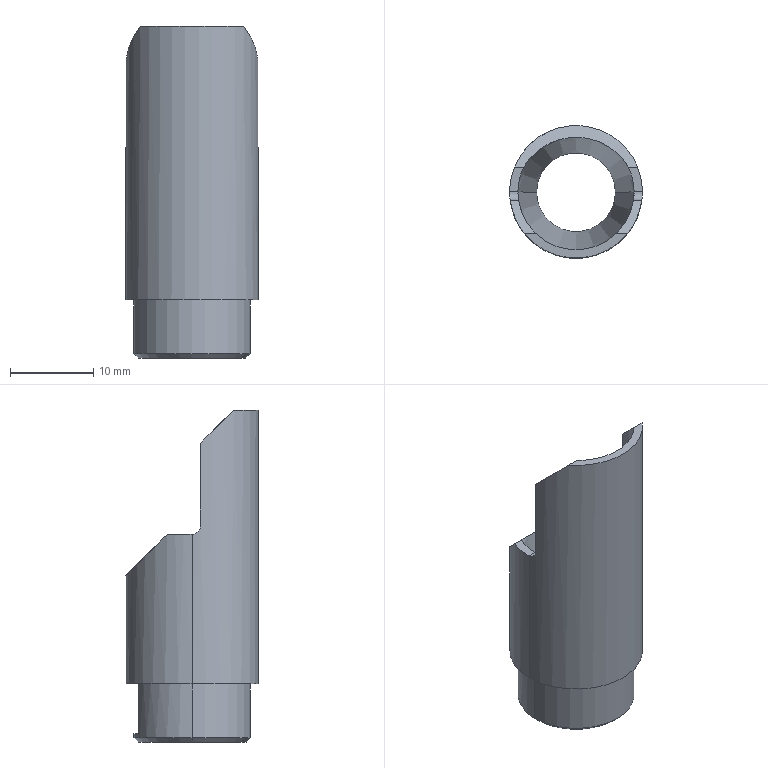Part | SolidWorks | features ICE 5, Chamfer 3, Extrusion 1, Fillet 1 | 1 solid | 25 faces | box 16 x 16 x 40 mm | volume 2380 mm3 | plane 12 | cylinder 9 | cone 4 | commonest cylinder face diameters 14 x3 2 x2 9.5 x2 16 x2
STEP:
#1=CARTESIAN_POINT('',(-4.75,0.,5.));
#2=VERTEX_POINT('',#1);
#3=CARTESIAN_POINT('',(4.75,0.,5.));
#4=VERTEX_POINT('',#3);
#5=CARTESIAN_POINT('',(0.,0.,5.));
#6=DIRECTION('',(0.,0.,1.));
#7=DIRECTION('',(1.,0.,0.));
#8=AXIS2_PLACEMENT_3D('',#5,#6,#7);
#9=CIRCLE('',#8,4.75);
#10=EDGE_CURVE('',#2,#4,#9,.T.);
#11=ORIENTED_EDGE('',*,*,#10,.F.);
#12=CARTESIAN_POINT('',(-7.,0.,25.));
#13=VERTEX_POINT('',#12);
#14=CARTESIAN_POINT('',(-4.75,0.,5.));
#15=DIRECTION('',(-0.1118,0.,0.9937));
#16=VECTOR('',#15,1000.);
#17=LINE('',#14,#16);
#18=EDGE_CURVE('',#2,#13,#17,.T.);
#19=ORIENTED_EDGE('',*,*,#18,.T.);
#20=CARTESIAN_POINT('',(7.,0.,25.));
#21=VERTEX_POINT('',#20);
#22=CARTESIAN_POINT('',(0.,0.,25.));
#23=DIRECTION('',(0.,0.,1.));
#24=DIRECTION('',(1.,0.,0.));
#25=AXIS2_PLACEMENT_3D('',#22,#23,#24);
#26=CIRCLE('',#25,7.);
#27=EDGE_CURVE('',#13,#21,#26,.T.);
#28=ORIENTED_EDGE('',*,*,#27,.T.);
#29=CARTESIAN_POINT('',(4.75,0.,5.));
#30=DIRECTION('',(0.1118,0.,0.9937));
#31=VECTOR('',#30,1000.);
#32=LINE('',#29,#31);
#33=EDGE_CURVE('',#4,#21,#32,.T.);
#34=ORIENTED_EDGE('',*,*,#33,.F.);
#35=EDGE_LOOP('',(#11,#19,#28,#34));
#36=FACE_OUTER_BOUND('',#35,.T.);
#37=CARTESIAN_POINT('',(0.,0.,5.));
#38=DIRECTION('',(0.,0.,1.));
#39=DIRECTION('',(1.,0.,0.));
#40=AXIS2_PLACEMENT_3D('',#37,#38,#39);
#41=CONICAL_SURFACE('',#40,4.75,0.112);
#42=ADVANCED_FACE('',(#36),#41,.F.);
#43=CARTESIAN_POINT('',(-6.5,0.,0.));
#44=VERTEX_POINT('',#43);
#45=CARTESIAN_POINT('',(6.5,0.,0.));
#46=VERTEX_POINT('',#45);
#47=CARTESIAN_POINT('',(0.,0.,0.));
#48=DIRECTION('',(0.,0.,-1.));
#49=DIRECTION('',(1.,0.,0.));
#50=AXIS2_PLACEMENT_3D('',#47,#48,#49);
#51=CIRCLE('',#50,6.5);
#52=EDGE_CURVE('',#44,#46,#51,.T.);
#53=ORIENTED_EDGE('',*,*,#52,.F.);
#54=CARTESIAN_POINT('',(-7.,0.,0.5));
#55=VERTEX_POINT('',#54);
#56=CARTESIAN_POINT('',(-6.5,0.,0.));
#57=DIRECTION('',(-0.7071,0.,0.7071));
#58=VECTOR('',#57,1000.);
#59=LINE('',#56,#58);
#60=EDGE_CURVE('',#44,#55,#59,.T.);
#61=ORIENTED_EDGE('',*,*,#60,.T.);
#62=CARTESIAN_POINT('',(7.,0.,0.5));
#63=VERTEX_POINT('',#62);
#64=CARTESIAN_POINT('',(0.,0.,0.5));
#65=DIRECTION('',(0.,0.,1.));
#66=DIRECTION('',(1.,0.,0.));
#67=AXIS2_PLACEMENT_3D('',#64,#65,#66);
#68=CIRCLE('',#67,7.);
#69=EDGE_CURVE('',#63,#55,#68,.T.);
#70=ORIENTED_EDGE('',*,*,#69,.F.);
#71=CARTESIAN_POINT('',(6.5,0.,0.));
#72=DIRECTION('',(0.7071,0.,0.7071));
#73=VECTOR('',#72,1000.);
#74=LINE('',#71,#73);
#75=EDGE_CURVE('',#46,#63,#74,.T.);
#76=ORIENTED_EDGE('',*,*,#75,.F.);
#77=EDGE_LOOP('',(#53,#61,#70,#76));
#78=FACE_OUTER_BOUND('',#77,.T.);
#79=CARTESIAN_POINT('',(0.,0.,0.));
#80=DIRECTION('',(0.,0.,1.));
#81=DIRECTION('',(1.,0.,0.));
#82=AXIS2_PLACEMENT_3D('',#79,#80,#81);
#83=CONICAL_SURFACE('',#82,6.5,0.7854);
#84=ADVANCED_FACE('',(#78),#83,.T.);
#85=CARTESIAN_POINT('',(7.416,3.,25.));
#86=VERTEX_POINT('',#85);
#87=CARTESIAN_POINT('',(8.,0.,25.));
#88=VERTEX_POINT('',#87);
#89=CARTESIAN_POINT('',(0.,0.,25.));
#90=DIRECTION('',(0.,0.,-1.));
#91=DIRECTION('',(-1.,0.,0.));
#92=AXIS2_PLACEMENT_3D('',#89,#90,#91);
#93=CIRCLE('',#92,8.);
#94=EDGE_CURVE('',#86,#88,#93,.T.);
#95=ORIENTED_EDGE('',*,*,#94,.T.);
#96=CARTESIAN_POINT('',(8.,0.,7.));
#97=VERTEX_POINT('',#96);
#98=CARTESIAN_POINT('',(8.,0.,40.));
#99=DIRECTION('',(0.,0.,-1.));
#100=VECTOR('',#99,1000.);
#101=LINE('',#98,#100);
#102=EDGE_CURVE('',#88,#97,#101,.T.);
#103=ORIENTED_EDGE('',*,*,#102,.T.);
#104=CARTESIAN_POINT('',(-8.,0.,7.));
#105=VERTEX_POINT('',#104);
#106=CARTESIAN_POINT('',(0.,0.,7.));
#107=DIRECTION('',(0.,0.,-1.));
#108=DIRECTION('',(-1.,0.,0.));
#109=AXIS2_PLACEMENT_3D('',#106,#107,#108);
#110=CIRCLE('',#109,8.);
#111=EDGE_CURVE('',#105,#97,#110,.T.);
#112=ORIENTED_EDGE('',*,*,#111,.F.);
#113=CARTESIAN_POINT('',(-8.,0.,25.));
#114=VERTEX_POINT('',#113);
#115=CARTESIAN_POINT('',(-8.,0.,40.));
#116=DIRECTION('',(0.,0.,-1.));
#117=VECTOR('',#116,1000.);
#118=LINE('',#115,#117);
#119=EDGE_CURVE('',#114,#105,#118,.T.);
#120=ORIENTED_EDGE('',*,*,#119,.F.);
#121=CARTESIAN_POINT('',(-7.416,3.,25.));
#122=VERTEX_POINT('',#121);
#123=CARTESIAN_POINT('',(0.,0.,25.));
#124=DIRECTION('',(0.,0.,-1.));
#125=DIRECTION('',(-1.,0.,0.));
#126=AXIS2_PLACEMENT_3D('',#123,#124,#125);
#127=CIRCLE('',#126,8.);
#128=EDGE_CURVE('',#114,#122,#127,.T.);
#129=ORIENTED_EDGE('',*,*,#128,.T.);
#130=CARTESIAN_POINT('',(-7.416,3.,25.));
#131=CARTESIAN_POINT('',(-4.238,10.857,17.143));
#132=CARTESIAN_POINT('',(4.238,10.857,17.143));
#133=CARTESIAN_POINT('',(7.416,3.,25.));
#134=(BOUNDED_CURVE()B_SPLINE_CURVE(3,(#130,#131,#132,#133),.UNSPECIFIED.,.F.,.F.)B_SPLINE_CURVE_WITH_KNOTS((4,4),(5.097,7.47),.UNSPECIFIED.)CURVE()GEOMETRIC_REPRESENTATION_ITEM()RATIONAL_B_SPLINE_CURVE((1.,0.5833,0.5833,1.))REPRESENTATION_ITEM(''));
#135=EDGE_CURVE('',#122,#86,#134,.T.);
#136=ORIENTED_EDGE('',*,*,#135,.T.);
#137=EDGE_LOOP('',(#95,#103,#112,#120,#129,#136));
#138=FACE_OUTER_BOUND('',#137,.T.);
#139=CARTESIAN_POINT('',(0.,0.,40.));
#140=DIRECTION('',(0.,0.,-1.));
#141=DIRECTION('',(-1.,0.,0.));
#142=AXIS2_PLACEMENT_3D('',#139,#140,#141);
#143=CYLINDRICAL_SURFACE('',#142,8.);
#144=ADVANCED_FACE('',(#138),#143,.T.);
#145=ORIENTED_EDGE('',*,*,#10,.T.);
#146=CARTESIAN_POINT('',(4.75,0.,0.));
#147=VERTEX_POINT('',#146);
#148=CARTESIAN_POINT('',(4.75,0.,40.));
#149=DIRECTION('',(0.,0.,-1.));
#150=VECTOR('',#149,1000.);
#151=LINE('',#148,#150);
#152=EDGE_CURVE('',#4,#147,#151,.T.);
#153=ORIENTED_EDGE('',*,*,#152,.T.);
#154=CARTESIAN_POINT('',(-4.75,0.,0.));
#155=VERTEX_POINT('',#154);
#156=CARTESIAN_POINT('',(0.,0.,0.));
#157=DIRECTION('',(0.,0.,1.));
#158=DIRECTION('',(1.,0.,0.));
#159=AXIS2_PLACEMENT_3D('',#156,#157,#158);
#160=CIRCLE('',#159,4.75);
#161=EDGE_CURVE('',#155,#147,#160,.T.);
#162=ORIENTED_EDGE('',*,*,#161,.F.);
#163=CARTESIAN_POINT('',(-4.75,0.,40.));
#164=DIRECTION('',(0.,0.,-1.));
#165=VECTOR('',#164,1000.);
#166=LINE('',#163,#165);
#167=EDGE_CURVE('',#2,#155,#166,.T.);
#168=ORIENTED_EDGE('',*,*,#167,.F.);
#169=EDGE_LOOP('',(#145,#153,#162,#168));
#170=FACE_OUTER_BOUND('',#169,.T.);
#171=CARTESIAN_POINT('',(0.,0.,40.));
#172=DIRECTION('',(0.,0.,-1.));
#173=DIRECTION('',(-1.,0.,0.));
#174=AXIS2_PLACEMENT_3D('',#171,#172,#173);
#175=CYLINDRICAL_SURFACE('',#174,4.75);
#176=ADVANCED_FACE('',(#170),#175,.F.);
#177=CARTESIAN_POINT('',(2.598,6.5,7.));
#178=VERTEX_POINT('',#177);
#179=CARTESIAN_POINT('',(7.,0.,7.));
#180=VERTEX_POINT('',#179);
#181=CARTESIAN_POINT('',(0.,0.,7.));
#182=DIRECTION('',(0.,0.,-1.));
#183=DIRECTION('',(-1.,0.,0.));
#184=AXIS2_PLACEMENT_3D('',#181,#182,#183);
#185=CIRCLE('',#184,7.);
#186=EDGE_CURVE('',#178,#180,#185,.T.);
#187=ORIENTED_EDGE('',*,*,#186,.T.);
#188=CARTESIAN_POINT('',(7.,0.,7.));
#189=DIRECTION('',(0.,0.,-1.));
#190=VECTOR('',#189,1000.);
#191=LINE('',#188,#190);
#192=EDGE_CURVE('',#180,#63,#191,.T.);
#193=ORIENTED_EDGE('',*,*,#192,.T.);
#194=ORIENTED_EDGE('',*,*,#69,.T.);
#195=CARTESIAN_POINT('',(-7.,0.,7.));
#196=VERTEX_POINT('',#195);
#197=CARTESIAN_POINT('',(-7.,0.,7.));
#198=DIRECTION('',(0.,0.,-1.));
#199=VECTOR('',#198,1000.);
#200=LINE('',#197,#199);
#201=EDGE_CURVE('',#196,#55,#200,.T.);
#202=ORIENTED_EDGE('',*,*,#201,.F.);
#203=CARTESIAN_POINT('',(-2.598,6.5,7.));
#204=VERTEX_POINT('',#203);
#205=CARTESIAN_POINT('',(0.,0.,7.));
#206=DIRECTION('',(0.,0.,-1.));
#207=DIRECTION('',(-1.,0.,0.));
#208=AXIS2_PLACEMENT_3D('',#205,#206,#207);
#209=CIRCLE('',#208,7.);
#210=EDGE_CURVE('',#196,#204,#209,.T.);
#211=ORIENTED_EDGE('',*,*,#210,.T.);
#212=CARTESIAN_POINT('',(-2.598,6.5,1.));
#213=VERTEX_POINT('',#212);
#214=CARTESIAN_POINT('',(-2.598,6.5,1.));
#215=DIRECTION('',(0.,0.,1.));
#216=VECTOR('',#215,1000.);
#217=LINE('',#214,#216);
#218=EDGE_CURVE('',#213,#204,#217,.T.);
#219=ORIENTED_EDGE('',*,*,#218,.F.);
#220=CARTESIAN_POINT('',(2.598,6.5,1.));
#221=VERTEX_POINT('',#220);
#222=CARTESIAN_POINT('',(0.,0.,1.));
#223=DIRECTION('',(0.,0.,-1.));
#224=DIRECTION('',(-1.,0.,0.));
#225=AXIS2_PLACEMENT_3D('',#222,#223,#224);
#226=CIRCLE('',#225,7.);
#227=EDGE_CURVE('',#213,#221,#226,.T.);
#228=ORIENTED_EDGE('',*,*,#227,.T.);
#229=CARTESIAN_POINT('',(2.598,6.5,1.));
#230=DIRECTION('',(0.,0.,1.));
#231=VECTOR('',#230,1000.);
#232=LINE('',#229,#231);
#233=EDGE_CURVE('',#221,#178,#232,.T.);
#234=ORIENTED_EDGE('',*,*,#233,.T.);
#235=EDGE_LOOP('',(#187,#193,#194,#202,#211,#219,#228,#234));
#236=FACE_OUTER_BOUND('',#235,.T.);
#237=CARTESIAN_POINT('',(0.,0.,7.));
#238=DIRECTION('',(0.,0.,-1.));
#239=DIRECTION('',(-1.,0.,0.));
#240=AXIS2_PLACEMENT_3D('',#237,#238,#239);
#241=CYLINDRICAL_SURFACE('',#240,7.);
#242=ADVANCED_FACE('',(#236),#241,.T.);
#243=ORIENTED_EDGE('',*,*,#192,.F.);
#244=CARTESIAN_POINT('',(0.,0.,7.));
#245=DIRECTION('',(0.,0.,-1.));
#246=DIRECTION('',(-1.,0.,0.));
#247=AXIS2_PLACEMENT_3D('',#244,#245,#246);
#248=CIRCLE('',#247,7.);
#249=EDGE_CURVE('',#180,#196,#248,.T.);
#250=ORIENTED_EDGE('',*,*,#249,.T.);
#251=ORIENTED_EDGE('',*,*,#201,.T.);
#252=CARTESIAN_POINT('',(0.,0.,0.5));
#253=DIRECTION('',(0.,0.,1.));
#254=DIRECTION('',(1.,0.,0.));
#255=AXIS2_PLACEMENT_3D('',#252,#253,#254);
#256=CIRCLE('',#255,7.);
#257=EDGE_CURVE('',#55,#63,#256,.T.);
#258=ORIENTED_EDGE('',*,*,#257,.T.);
#259=EDGE_LOOP('',(#243,#250,#251,#258));
#260=FACE_OUTER_BOUND('',#259,.T.);
#261=CARTESIAN_POINT('',(0.,0.,7.));
#262=DIRECTION('',(0.,0.,-1.));
#263=DIRECTION('',(-1.,0.,0.));
#264=AXIS2_PLACEMENT_3D('',#261,#262,#263);
#265=CYLINDRICAL_SURFACE('',#264,7.);
#266=ADVANCED_FACE('',(#260),#265,.T.);
#267=ORIENTED_EDGE('',*,*,#128,.F.);
#268=CARTESIAN_POINT('',(0.,0.,25.));
#269=DIRECTION('',(1.,0.,0.));
#270=VECTOR('',#269,1000.);
#271=LINE('',#268,#270);
#272=EDGE_CURVE('',#114,#13,#271,.T.);
#273=ORIENTED_EDGE('',*,*,#272,.T.);
#274=CARTESIAN_POINT('',(-6.325,3.,25.));
#275=VERTEX_POINT('',#274);
#276=CARTESIAN_POINT('',(0.,0.,25.));
#277=DIRECTION('',(0.,0.,-1.));
#278=DIRECTION('',(1.,0.,0.));
#279=AXIS2_PLACEMENT_3D('',#276,#277,#278);
#280=CIRCLE('',#279,7.);
#281=EDGE_CURVE('',#13,#275,#280,.T.);
#282=ORIENTED_EDGE('',*,*,#281,.T.);
#283=CARTESIAN_POINT('',(-8.,3.,25.));
#284=DIRECTION('',(1.,0.,0.));
#285=VECTOR('',#284,1000.);
#286=LINE('',#283,#285);
#287=EDGE_CURVE('',#122,#275,#286,.T.);
#288=ORIENTED_EDGE('',*,*,#287,.F.);
#289=EDGE_LOOP('',(#267,#273,#282,#288));
#290=FACE_OUTER_BOUND('',#289,.T.);
#291=CARTESIAN_POINT('',(0.,0.,25.));
#292=DIRECTION('',(0.,0.,1.));
#293=DIRECTION('',(1.,0.,0.));
#294=AXIS2_PLACEMENT_3D('',#291,#292,#293);
#295=PLANE('',#294);
#296=ADVANCED_FACE('',(#290),#295,.T.);
#297=ORIENTED_EDGE('',*,*,#152,.F.);
#298=CARTESIAN_POINT('',(0.,0.,5.));
#299=DIRECTION('',(0.,0.,1.));
#300=DIRECTION('',(1.,0.,0.));
#301=AXIS2_PLACEMENT_3D('',#298,#299,#300);
#302=CIRCLE('',#301,4.75);
#303=EDGE_CURVE('',#4,#2,#302,.T.);
#304=ORIENTED_EDGE('',*,*,#303,.T.);
#305=ORIENTED_EDGE('',*,*,#167,.T.);
#306=CARTESIAN_POINT('',(0.,0.,0.));
#307=DIRECTION('',(0.,0.,1.));
#308=DIRECTION('',(1.,0.,0.));
#309=AXIS2_PLACEMENT_3D('',#306,#307,#308);
#310=CIRCLE('',#309,4.75);
#311=EDGE_CURVE('',#147,#155,#310,.T.);
#312=ORIENTED_EDGE('',*,*,#311,.F.);
#313=EDGE_LOOP('',(#297,#304,#305,#312));
#314=FACE_OUTER_BOUND('',#313,.T.);
#315=CARTESIAN_POINT('',(0.,0.,40.));
#316=DIRECTION('',(0.,0.,-1.));
#317=DIRECTION('',(-1.,0.,0.));
#318=AXIS2_PLACEMENT_3D('',#315,#316,#317);
#319=CYLINDRICAL_SURFACE('',#318,4.75);
#320=ADVANCED_FACE('',(#314),#319,.F.);
#321=CARTESIAN_POINT('',(0.,0.,0.));
#322=DIRECTION('',(0.,0.,-1.));
#323=DIRECTION('',(1.,0.,0.));
#324=AXIS2_PLACEMENT_3D('',#321,#322,#323);
#325=CIRCLE('',#324,6.5);
#326=EDGE_CURVE('',#46,#44,#325,.T.);
#327=ORIENTED_EDGE('',*,*,#326,.T.);
#328=ORIENTED_EDGE('',*,*,#52,.T.);
#329=EDGE_LOOP('',(#327,#328));
#330=FACE_OUTER_BOUND('',#329,.T.);
#331=ORIENTED_EDGE('',*,*,#161,.T.);
#332=ORIENTED_EDGE('',*,*,#311,.T.);
#333=EDGE_LOOP('',(#331,#332));
#334=FACE_BOUND('',#333,.T.);
#335=CARTESIAN_POINT('',(0.,0.,0.));
#336=DIRECTION('',(0.,0.,1.));
#337=DIRECTION('',(1.,0.,0.));
#338=AXIS2_PLACEMENT_3D('',#335,#336,#337);
#339=PLANE('',#338);
#340=ADVANCED_FACE('',(#330,#334),#339,.F.);
#341=ORIENTED_EDGE('',*,*,#102,.F.);
#342=CARTESIAN_POINT('',(7.937,-1.,26.));
#343=VERTEX_POINT('',#342);
#344=CARTESIAN_POINT('',(8.,0.,25.));
#345=CARTESIAN_POINT('',(8.,-0.1322,25.));
#346=CARTESIAN_POINT('',(7.997,-0.2619,25.026));
#347=CARTESIAN_POINT('',(7.985,-0.5039,25.126));
#348=CARTESIAN_POINT('',(7.977,-0.6147,25.201));
#349=CARTESIAN_POINT('',(7.952,-0.8911,25.477));
#350=CARTESIAN_POINT('',(7.937,-1.,25.736));
#351=CARTESIAN_POINT('',(7.937,-1.,26.));
#352=B_SPLINE_CURVE_WITH_KNOTS('',3,(#344,#345,#346,#347,#348,#349,#350,#351),.UNSPECIFIED.,.F.,.F.,(4,2,2,4),(0.,0.0003909,0.0007818,0.001564),.UNSPECIFIED.);
#353=EDGE_CURVE('',#88,#343,#352,.T.);
#354=ORIENTED_EDGE('',*,*,#353,.T.);
#355=CARTESIAN_POINT('',(7.937,-1.,36.));
#356=VERTEX_POINT('',#355);
#357=CARTESIAN_POINT('',(7.937,-1.,40.));
#358=DIRECTION('',(0.,0.,1.));
#359=VECTOR('',#358,1000.);
#360=LINE('',#357,#359);
#361=EDGE_CURVE('',#343,#356,#360,.T.);
#362=ORIENTED_EDGE('',*,*,#361,.T.);
#363=CARTESIAN_POINT('',(6.245,-5.,40.));
#364=VERTEX_POINT('',#363);
#365=CARTESIAN_POINT('',(7.937,-1.,36.));
#366=CARTESIAN_POINT('',(7.752,-2.473,37.473));
#367=CARTESIAN_POINT('',(7.173,-3.841,38.841));
#368=CARTESIAN_POINT('',(6.245,-5.,40.));
#369=(BOUNDED_CURVE()B_SPLINE_CURVE(3,(#365,#366,#367,#368),.UNSPECIFIED.,.F.,.F.)B_SPLINE_CURVE_WITH_KNOTS((4,4),(1.696,2.246),.UNSPECIFIED.)CURVE()GEOMETRIC_REPRESENTATION_ITEM()RATIONAL_B_SPLINE_CURVE((1.,0.975,0.975,1.))REPRESENTATION_ITEM(''));
#370=EDGE_CURVE('',#356,#364,#369,.T.);
#371=ORIENTED_EDGE('',*,*,#370,.T.);
#372=CARTESIAN_POINT('',(-6.245,-5.,40.));
#373=VERTEX_POINT('',#372);
#374=CARTESIAN_POINT('',(0.,0.,40.));
#375=DIRECTION('',(0.,0.,1.));
#376=DIRECTION('',(1.,0.,0.));
#377=AXIS2_PLACEMENT_3D('',#374,#375,#376);
#378=CIRCLE('',#377,8.);
#379=EDGE_CURVE('',#373,#364,#378,.T.);
#380=ORIENTED_EDGE('',*,*,#379,.F.);
#381=CARTESIAN_POINT('',(-7.937,-1.,36.));
#382=VERTEX_POINT('',#381);
#383=CARTESIAN_POINT('',(-6.245,-5.,40.));
#384=CARTESIAN_POINT('',(-7.173,-3.841,38.841));
#385=CARTESIAN_POINT('',(-7.752,-2.473,37.473));
#386=CARTESIAN_POINT('',(-7.937,-1.,36.));
#387=(BOUNDED_CURVE()B_SPLINE_CURVE(3,(#383,#384,#385,#386),.UNSPECIFIED.,.F.,.F.)B_SPLINE_CURVE_WITH_KNOTS((4,4),(4.037,4.587),.UNSPECIFIED.)CURVE()GEOMETRIC_REPRESENTATION_ITEM()RATIONAL_B_SPLINE_CURVE((1.,0.975,0.975,1.))REPRESENTATION_ITEM(''));
#388=EDGE_CURVE('',#373,#382,#387,.T.);
#389=ORIENTED_EDGE('',*,*,#388,.T.);
#390=CARTESIAN_POINT('',(-7.937,-1.,26.));
#391=VERTEX_POINT('',#390);
#392=CARTESIAN_POINT('',(-7.937,-1.,40.));
#393=DIRECTION('',(0.,0.,-1.));
#394=VECTOR('',#393,1000.);
#395=LINE('',#392,#394);
#396=EDGE_CURVE('',#382,#391,#395,.T.);
#397=ORIENTED_EDGE('',*,*,#396,.T.);
#398=CARTESIAN_POINT('',(-7.937,-1.,26.));
#399=CARTESIAN_POINT('',(-7.937,-1.,25.868));
#400=CARTESIAN_POINT('',(-7.941,-0.9739,25.738));
#401=CARTESIAN_POINT('',(-7.952,-0.8736,25.496));
#402=CARTESIAN_POINT('',(-7.96,-0.7994,25.385));
#403=CARTESIAN_POINT('',(-7.985,-0.5232,25.109));
#404=CARTESIAN_POINT('',(-8.,-0.2644,25.));
#405=CARTESIAN_POINT('',(-8.,0.,25.));
#406=B_SPLINE_CURVE_WITH_KNOTS('',3,(#398,#399,#400,#401,#402,#403,#404,#405),.UNSPECIFIED.,.F.,.F.,(4,2,2,4),(0.,0.0003909,0.0007818,0.001564),.UNSPECIFIED.);
#407=EDGE_CURVE('',#391,#114,#406,.T.);
#408=ORIENTED_EDGE('',*,*,#407,.T.);
#409=ORIENTED_EDGE('',*,*,#119,.T.);
#410=CARTESIAN_POINT('',(0.,0.,7.));
#411=DIRECTION('',(0.,0.,-1.));
#412=DIRECTION('',(-1.,0.,0.));
#413=AXIS2_PLACEMENT_3D('',#410,#411,#412);
#414=CIRCLE('',#413,8.);
#415=EDGE_CURVE('',#97,#105,#414,.T.);
#416=ORIENTED_EDGE('',*,*,#415,.F.);
#417=EDGE_LOOP('',(#341,#354,#362,#371,#380,#389,#397,#408,#409,#416));
#418=FACE_OUTER_BOUND('',#417,.T.);
#419=CARTESIAN_POINT('',(0.,0.,40.));
#420=DIRECTION('',(0.,0.,-1.));
#421=DIRECTION('',(-1.,0.,0.));
#422=AXIS2_PLACEMENT_3D('',#419,#420,#421);
#423=CYLINDRICAL_SURFACE('',#422,8.);
#424=ADVANCED_FACE('',(#418),#423,.T.);
#425=ORIENTED_EDGE('',*,*,#379,.T.);
#426=CARTESIAN_POINT('',(4.899,-5.,40.));
#427=VERTEX_POINT('',#426);
#428=CARTESIAN_POINT('',(6.928,-5.,40.));
#429=DIRECTION('',(-1.,0.,0.));
#430=VECTOR('',#429,1000.);
#431=LINE('',#428,#430);
#432=EDGE_CURVE('',#364,#427,#431,.T.);
#433=ORIENTED_EDGE('',*,*,#432,.T.);
#434=CARTESIAN_POINT('',(-4.899,-5.,40.));
#435=VERTEX_POINT('',#434);
#436=CARTESIAN_POINT('',(0.,0.,40.));
#437=DIRECTION('',(0.,0.,1.));
#438=DIRECTION('',(1.,0.,0.));
#439=AXIS2_PLACEMENT_3D('',#436,#437,#438);
#440=CIRCLE('',#439,7.);
#441=EDGE_CURVE('',#435,#427,#440,.T.);
#442=ORIENTED_EDGE('',*,*,#441,.F.);
#443=CARTESIAN_POINT('',(-7.937,-5.,40.));
#444=DIRECTION('',(-1.,0.,0.));
#445=VECTOR('',#444,1000.);
#446=LINE('',#443,#445);
#447=EDGE_CURVE('',#435,#373,#446,.T.);
#448=ORIENTED_EDGE('',*,*,#447,.T.);
#449=EDGE_LOOP('',(#425,#433,#442,#448));
#450=FACE_OUTER_BOUND('',#449,.T.);
#451=CARTESIAN_POINT('',(0.,0.,40.));
#452=DIRECTION('',(0.,0.,1.));
#453=DIRECTION('',(1.,0.,0.));
#454=AXIS2_PLACEMENT_3D('',#451,#452,#453);
#455=PLANE('',#454);
#456=ADVANCED_FACE('',(#450),#455,.T.);
#457=ORIENTED_EDGE('',*,*,#186,.F.);
#458=CARTESIAN_POINT('',(2.598,6.5,7.));
#459=DIRECTION('',(-1.,0.,0.));
#460=VECTOR('',#459,1000.);
#461=LINE('',#458,#460);
#462=EDGE_CURVE('',#178,#204,#461,.T.);
#463=ORIENTED_EDGE('',*,*,#462,.T.);
#464=ORIENTED_EDGE('',*,*,#210,.F.);
#465=ORIENTED_EDGE('',*,*,#249,.F.);
#466=EDGE_LOOP('',(#457,#463,#464,#465));
#467=FACE_BOUND('',#466,.T.);
#468=ORIENTED_EDGE('',*,*,#111,.T.);
#469=ORIENTED_EDGE('',*,*,#415,.T.);
#470=EDGE_LOOP('',(#468,#469));
#471=FACE_OUTER_BOUND('',#470,.T.);
#472=CARTESIAN_POINT('',(0.,0.,7.));
#473=DIRECTION('',(0.,0.,-1.));
#474=DIRECTION('',(-1.,0.,0.));
#475=AXIS2_PLACEMENT_3D('',#472,#473,#474);
#476=PLANE('',#475);
#477=ADVANCED_FACE('',(#467,#471),#476,.T.);
#478=ORIENTED_EDGE('',*,*,#60,.F.);
#479=ORIENTED_EDGE('',*,*,#326,.F.);
#480=ORIENTED_EDGE('',*,*,#75,.T.);
#481=ORIENTED_EDGE('',*,*,#257,.F.);
#482=EDGE_LOOP('',(#478,#479,#480,#481));
#483=FACE_OUTER_BOUND('',#482,.T.);
#484=CARTESIAN_POINT('',(0.,0.,0.));
#485=DIRECTION('',(0.,0.,1.));
#486=DIRECTION('',(1.,0.,0.));
#487=AXIS2_PLACEMENT_3D('',#484,#485,#486);
#488=CONICAL_SURFACE('',#487,6.5,0.7854);
#489=ADVANCED_FACE('',(#483),#488,.T.);
#490=ORIENTED_EDGE('',*,*,#441,.T.);
#491=CARTESIAN_POINT('',(6.928,-1.,36.));
#492=VERTEX_POINT('',#491);
#493=CARTESIAN_POINT('',(4.899,-5.,40.));
#494=CARTESIAN_POINT('',(6.006,-3.916,38.916));
#495=CARTESIAN_POINT('',(6.707,-2.534,37.534));
#496=CARTESIAN_POINT('',(6.928,-1.,36.));
#497=(BOUNDED_CURVE()B_SPLINE_CURVE(3,(#493,#494,#495,#496),.UNSPECIFIED.,.F.,.F.)B_SPLINE_CURVE_WITH_KNOTS((4,4),(0.7752,1.427),.UNSPECIFIED.)CURVE()GEOMETRIC_REPRESENTATION_ITEM()RATIONAL_B_SPLINE_CURVE((1.,0.9649,0.9649,1.))REPRESENTATION_ITEM(''));
#498=EDGE_CURVE('',#427,#492,#497,.T.);
#499=ORIENTED_EDGE('',*,*,#498,.T.);
#500=CARTESIAN_POINT('',(6.928,-1.,26.));
#501=VERTEX_POINT('',#500);
#502=CARTESIAN_POINT('',(6.928,-1.,25.));
#503=DIRECTION('',(0.,0.,-1.));
#504=VECTOR('',#503,1000.);
#505=LINE('',#502,#504);
#506=EDGE_CURVE('',#492,#501,#505,.T.);
#507=ORIENTED_EDGE('',*,*,#506,.T.);
#508=CARTESIAN_POINT('',(6.928,-1.,26.));
#509=CARTESIAN_POINT('',(6.928,-1.,25.868));
#510=CARTESIAN_POINT('',(6.932,-0.9739,25.738));
#511=CARTESIAN_POINT('',(6.945,-0.8736,25.496));
#512=CARTESIAN_POINT('',(6.955,-0.7994,25.385));
#513=CARTESIAN_POINT('',(6.983,-0.5233,25.109));
#514=CARTESIAN_POINT('',(7.,-0.2645,25.));
#515=CARTESIAN_POINT('',(7.,0.,25.));
#516=B_SPLINE_CURVE_WITH_KNOTS('',3,(#508,#509,#510,#511,#512,#513,#514,#515),.UNSPECIFIED.,.F.,.F.,(4,2,2,4),(0.,0.000391,0.0007821,0.001564),.UNSPECIFIED.);
#517=EDGE_CURVE('',#501,#21,#516,.T.);
#518=ORIENTED_EDGE('',*,*,#517,.T.);
#519=ORIENTED_EDGE('',*,*,#27,.F.);
#520=CARTESIAN_POINT('',(-6.928,-1.,26.));
#521=VERTEX_POINT('',#520);
#522=CARTESIAN_POINT('',(-7.,0.,25.));
#523=CARTESIAN_POINT('',(-7.,-0.1322,25.));
#524=CARTESIAN_POINT('',(-6.996,-0.262,25.026));
#525=CARTESIAN_POINT('',(-6.983,-0.504,25.126));
#526=CARTESIAN_POINT('',(-6.974,-0.6148,25.201));
#527=CARTESIAN_POINT('',(-6.946,-0.8911,25.477));
#528=CARTESIAN_POINT('',(-6.928,-1.,25.736));
#529=CARTESIAN_POINT('',(-6.928,-1.,26.));
#530=B_SPLINE_CURVE_WITH_KNOTS('',3,(#522,#523,#524,#525,#526,#527,#528,#529),.UNSPECIFIED.,.F.,.F.,(4,2,2,4),(0.,0.000391,0.0007821,0.001564),.UNSPECIFIED.);
#531=EDGE_CURVE('',#13,#521,#530,.T.);
#532=ORIENTED_EDGE('',*,*,#531,.T.);
#533=CARTESIAN_POINT('',(-6.928,-1.,36.));
#534=VERTEX_POINT('',#533);
#535=CARTESIAN_POINT('',(-6.928,-1.,25.));
#536=DIRECTION('',(0.,0.,1.));
#537=VECTOR('',#536,1000.);
#538=LINE('',#535,#537);
#539=EDGE_CURVE('',#521,#534,#538,.T.);
#540=ORIENTED_EDGE('',*,*,#539,.T.);
#541=CARTESIAN_POINT('',(-6.928,-1.,36.));
#542=CARTESIAN_POINT('',(-6.707,-2.534,37.534));
#543=CARTESIAN_POINT('',(-6.006,-3.916,38.916));
#544=CARTESIAN_POINT('',(-4.899,-5.,40.));
#545=(BOUNDED_CURVE()B_SPLINE_CURVE(3,(#541,#542,#543,#544),.UNSPECIFIED.,.F.,.F.)B_SPLINE_CURVE_WITH_KNOTS((4,4),(4.856,5.508),.UNSPECIFIED.)CURVE()GEOMETRIC_REPRESENTATION_ITEM()RATIONAL_B_SPLINE_CURVE((1.,0.9649,0.9649,1.))REPRESENTATION_ITEM(''));
#546=EDGE_CURVE('',#534,#435,#545,.T.);
#547=ORIENTED_EDGE('',*,*,#546,.T.);
#548=EDGE_LOOP('',(#490,#499,#507,#518,#519,#532,#540,#547));
#549=FACE_OUTER_BOUND('',#548,.T.);
#550=CARTESIAN_POINT('',(0.,0.,25.));
#551=DIRECTION('',(0.,0.,1.));
#552=DIRECTION('',(1.,0.,0.));
#553=AXIS2_PLACEMENT_3D('',#550,#551,#552);
#554=CYLINDRICAL_SURFACE('',#553,7.);
#555=ADVANCED_FACE('',(#549),#554,.F.);
#556=CARTESIAN_POINT('',(6.325,3.,25.));
#557=VERTEX_POINT('',#556);
#558=CARTESIAN_POINT('',(0.,0.,25.));
#559=DIRECTION('',(0.,0.,-1.));
#560=DIRECTION('',(1.,0.,0.));
#561=AXIS2_PLACEMENT_3D('',#558,#559,#560);
#562=CIRCLE('',#561,7.);
#563=EDGE_CURVE('',#557,#21,#562,.T.);
#564=ORIENTED_EDGE('',*,*,#563,.T.);
#565=CARTESIAN_POINT('',(0.,0.,25.));
#566=DIRECTION('',(1.,0.,0.));
#567=VECTOR('',#566,1000.);
#568=LINE('',#565,#567);
#569=EDGE_CURVE('',#21,#88,#568,.T.);
#570=ORIENTED_EDGE('',*,*,#569,.T.);
#571=ORIENTED_EDGE('',*,*,#94,.F.);
#572=CARTESIAN_POINT('',(-8.,3.,25.));
#573=DIRECTION('',(1.,0.,0.));
#574=VECTOR('',#573,1000.);
#575=LINE('',#572,#574);
#576=EDGE_CURVE('',#557,#86,#575,.T.);
#577=ORIENTED_EDGE('',*,*,#576,.F.);
#578=EDGE_LOOP('',(#564,#570,#571,#577));
#579=FACE_OUTER_BOUND('',#578,.T.);
#580=CARTESIAN_POINT('',(0.,0.,25.));
#581=DIRECTION('',(0.,0.,1.));
#582=DIRECTION('',(1.,0.,0.));
#583=AXIS2_PLACEMENT_3D('',#580,#581,#582);
#584=PLANE('',#583);
#585=ADVANCED_FACE('',(#579),#584,.T.);
#586=ORIENTED_EDGE('',*,*,#539,.F.);
#587=CARTESIAN_POINT('',(-8.,-1.,26.));
#588=DIRECTION('',(-1.,0.,0.));
#589=VECTOR('',#588,1000.);
#590=LINE('',#587,#589);
#591=EDGE_CURVE('',#521,#391,#590,.T.);
#592=ORIENTED_EDGE('',*,*,#591,.T.);
#593=ORIENTED_EDGE('',*,*,#396,.F.);
#594=CARTESIAN_POINT('',(-6.928,-1.,36.));
#595=DIRECTION('',(1.,0.,0.));
#596=VECTOR('',#595,1000.);
#597=LINE('',#594,#596);
#598=EDGE_CURVE('',#382,#534,#597,.T.);
#599=ORIENTED_EDGE('',*,*,#598,.T.);
#600=EDGE_LOOP('',(#586,#592,#593,#599));
#601=FACE_OUTER_BOUND('',#600,.T.);
#602=CARTESIAN_POINT('',(-8.,-1.,40.));
#603=DIRECTION('',(0.,-1.,0.));
#604=DIRECTION('',(0.,0.,-1.));
#605=AXIS2_PLACEMENT_3D('',#602,#603,#604);
#606=PLANE('',#605);
#607=ADVANCED_FACE('',(#601),#606,.F.);
#608=ORIENTED_EDGE('',*,*,#361,.F.);
#609=CARTESIAN_POINT('',(-8.,-1.,26.));
#610=DIRECTION('',(-1.,0.,0.));
#611=VECTOR('',#610,1000.);
#612=LINE('',#609,#611);
#613=EDGE_CURVE('',#343,#501,#612,.T.);
#614=ORIENTED_EDGE('',*,*,#613,.T.);
#615=ORIENTED_EDGE('',*,*,#506,.F.);
#616=CARTESIAN_POINT('',(7.937,-1.,36.));
#617=DIRECTION('',(1.,0.,0.));
#618=VECTOR('',#617,1000.);
#619=LINE('',#616,#618);
#620=EDGE_CURVE('',#492,#356,#619,.T.);
#621=ORIENTED_EDGE('',*,*,#620,.T.);
#622=EDGE_LOOP('',(#608,#614,#615,#621));
#623=FACE_OUTER_BOUND('',#622,.T.);
#624=CARTESIAN_POINT('',(-8.,-1.,40.));
#625=DIRECTION('',(0.,-1.,0.));
#626=DIRECTION('',(0.,0.,-1.));
#627=AXIS2_PLACEMENT_3D('',#624,#625,#626);
#628=PLANE('',#627);
#629=ADVANCED_FACE('',(#623),#628,.F.);
#630=ORIENTED_EDGE('',*,*,#18,.F.);
#631=ORIENTED_EDGE('',*,*,#303,.F.);
#632=ORIENTED_EDGE('',*,*,#33,.T.);
#633=ORIENTED_EDGE('',*,*,#563,.F.);
#634=CARTESIAN_POINT('',(-6.325,3.,25.));
#635=CARTESIAN_POINT('',(-3.112,8.365,19.635));
#636=CARTESIAN_POINT('',(3.112,8.365,19.635));
#637=CARTESIAN_POINT('',(6.325,3.,25.));
#638=(BOUNDED_CURVE()B_SPLINE_CURVE(3,(#634,#635,#636,#637),.UNSPECIFIED.,.F.,.F.)B_SPLINE_CURVE_WITH_KNOTS((4,4),(2.113,4.17),.UNSPECIFIED.)CURVE()GEOMETRIC_REPRESENTATION_ITEM()RATIONAL_B_SPLINE_CURVE((1.,0.6775,0.6775,1.))REPRESENTATION_ITEM(''));
#639=EDGE_CURVE('',#275,#557,#638,.T.);
#640=ORIENTED_EDGE('',*,*,#639,.F.);
#641=ORIENTED_EDGE('',*,*,#281,.F.);
#642=EDGE_LOOP('',(#630,#631,#632,#633,#640,#641));
#643=FACE_OUTER_BOUND('',#642,.T.);
#644=CARTESIAN_POINT('',(0.,0.,5.));
#645=DIRECTION('',(0.,0.,1.));
#646=DIRECTION('',(1.,0.,0.));
#647=AXIS2_PLACEMENT_3D('',#644,#645,#646);
#648=CONICAL_SURFACE('',#647,4.75,0.112);
#649=ADVANCED_FACE('',(#643),#648,.F.);
#650=ORIENTED_EDGE('',*,*,#498,.F.);
#651=ORIENTED_EDGE('',*,*,#432,.F.);
#652=ORIENTED_EDGE('',*,*,#370,.F.);
#653=ORIENTED_EDGE('',*,*,#620,.F.);
#654=EDGE_LOOP('',(#650,#651,#652,#653));
#655=FACE_OUTER_BOUND('',#654,.T.);
#656=CARTESIAN_POINT('',(-8.,-1.,36.));
#657=DIRECTION('',(0.,0.7071,0.7071));
#658=DIRECTION('',(-1.,0.,0.));
#659=AXIS2_PLACEMENT_3D('',#656,#657,#658);
#660=PLANE('',#659);
#661=ADVANCED_FACE('',(#655),#660,.T.);
#662=ORIENTED_EDGE('',*,*,#388,.F.);
#663=ORIENTED_EDGE('',*,*,#447,.F.);
#664=ORIENTED_EDGE('',*,*,#546,.F.);
#665=ORIENTED_EDGE('',*,*,#598,.F.);
#666=EDGE_LOOP('',(#662,#663,#664,#665));
#667=FACE_OUTER_BOUND('',#666,.T.);
#668=CARTESIAN_POINT('',(-8.,-1.,36.));
#669=DIRECTION('',(0.,0.7071,0.7071));
#670=DIRECTION('',(-1.,0.,0.));
#671=AXIS2_PLACEMENT_3D('',#668,#669,#670);
#672=PLANE('',#671);
#673=ADVANCED_FACE('',(#667),#672,.T.);
#674=ORIENTED_EDGE('',*,*,#135,.F.);
#675=ORIENTED_EDGE('',*,*,#287,.T.);
#676=ORIENTED_EDGE('',*,*,#639,.T.);
#677=ORIENTED_EDGE('',*,*,#576,.T.);
#678=EDGE_LOOP('',(#674,#675,#676,#677));
#679=FACE_OUTER_BOUND('',#678,.T.);
#680=CARTESIAN_POINT('',(-8.,8.,20.));
#681=DIRECTION('',(0.,-0.7071,-0.7071));
#682=DIRECTION('',(0.,0.7071,-0.7071));
#683=AXIS2_PLACEMENT_3D('',#680,#681,#682);
#684=PLANE('',#683);
#685=ADVANCED_FACE('',(#679),#684,.F.);
#686=ORIENTED_EDGE('',*,*,#517,.F.);
#687=ORIENTED_EDGE('',*,*,#613,.F.);
#688=ORIENTED_EDGE('',*,*,#353,.F.);
#689=ORIENTED_EDGE('',*,*,#569,.F.);
#690=EDGE_LOOP('',(#686,#687,#688,#689));
#691=FACE_OUTER_BOUND('',#690,.T.);
#692=CARTESIAN_POINT('',(0.,0.,26.));
#693=DIRECTION('',(1.,0.,0.));
#694=DIRECTION('',(0.,0.,-1.));
#695=AXIS2_PLACEMENT_3D('',#692,#693,#694);
#696=CYLINDRICAL_SURFACE('',#695,1.);
#697=ADVANCED_FACE('',(#691),#696,.F.);
#698=ORIENTED_EDGE('',*,*,#407,.F.);
#699=ORIENTED_EDGE('',*,*,#591,.F.);
#700=ORIENTED_EDGE('',*,*,#531,.F.);
#701=ORIENTED_EDGE('',*,*,#272,.F.);
#702=EDGE_LOOP('',(#698,#699,#700,#701));
#703=FACE_OUTER_BOUND('',#702,.T.);
#704=CARTESIAN_POINT('',(0.,0.,26.));
#705=DIRECTION('',(1.,0.,0.));
#706=DIRECTION('',(0.,0.,-1.));
#707=AXIS2_PLACEMENT_3D('',#704,#705,#706);
#708=CYLINDRICAL_SURFACE('',#707,1.);
#709=ADVANCED_FACE('',(#703),#708,.F.);
#710=ORIENTED_EDGE('',*,*,#462,.F.);
#711=ORIENTED_EDGE('',*,*,#233,.F.);
#712=CARTESIAN_POINT('',(2.598,6.5,1.));
#713=DIRECTION('',(-1.,0.,0.));
#714=VECTOR('',#713,1000.);
#715=LINE('',#712,#714);
#716=EDGE_CURVE('',#221,#213,#715,.T.);
#717=ORIENTED_EDGE('',*,*,#716,.T.);
#718=ORIENTED_EDGE('',*,*,#218,.T.);
#719=EDGE_LOOP('',(#710,#711,#717,#718));
#720=FACE_OUTER_BOUND('',#719,.T.);
#721=CARTESIAN_POINT('',(2.598,6.5,1.));
#722=DIRECTION('',(0.,1.,0.));
#723=DIRECTION('',(0.,0.,1.));
#724=AXIS2_PLACEMENT_3D('',#721,#722,#723);
#725=PLANE('',#724);
#726=ADVANCED_FACE('',(#720),#725,.T.);
#727=ORIENTED_EDGE('',*,*,#227,.F.);
#728=ORIENTED_EDGE('',*,*,#716,.F.);
#729=EDGE_LOOP('',(#727,#728));
#730=FACE_OUTER_BOUND('',#729,.T.);
#731=CARTESIAN_POINT('',(0.,0.,1.));
#732=DIRECTION('',(0.,0.,-1.));
#733=DIRECTION('',(-1.,0.,0.));
#734=AXIS2_PLACEMENT_3D('',#731,#732,#733);
#735=PLANE('',#734);
#736=ADVANCED_FACE('',(#730),#735,.F.);
#737=CLOSED_SHELL('',(#42,#84,#144,#176,#242,#266,#296,#320,#340,#424,#456,#477,#489,#555,#585,#607,#629,#649,#661,#673,#685,#697,#709,#726,#736));
#738=MANIFOLD_SOLID_BREP('',#737);
#739=CARTESIAN_POINT('',(0.,0.,0.));
#740=DIRECTION('',(0.,0.,1.));
#741=DIRECTION('',(1.,0.,0.));
#742=AXIS2_PLACEMENT_3D('',#739,#740,#741);
#743=(LENGTH_UNIT()NAMED_UNIT(*)SI_UNIT(.MILLI.,.METRE.));
#744=UNCERTAINTY_MEASURE_WITH_UNIT(LENGTH_MEASURE(0.00001),#743,'','');
#745=(NAMED_UNIT(*)PLANE_ANGLE_UNIT()SI_UNIT($,.RADIAN.));
#746=(NAMED_UNIT(*)SI_UNIT($,.STERADIAN.)SOLID_ANGLE_UNIT());
#747=(GEOMETRIC_REPRESENTATION_CONTEXT(3)GLOBAL_UNCERTAINTY_ASSIGNED_CONTEXT((#744))GLOBAL_UNIT_ASSIGNED_CONTEXT((#743,#745,#746))REPRESENTATION_CONTEXT('',''));
#748=ADVANCED_BREP_SHAPE_REPRESENTATION('',(#738,#742),#747);